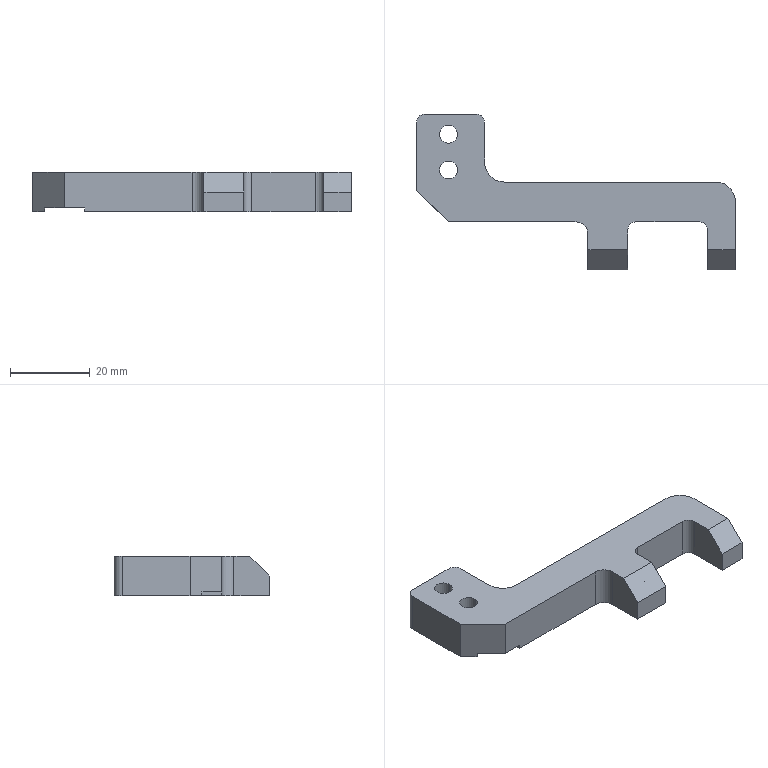Part | STEP file | PN_0045 | 1 solid | 48 faces | box 80 x 39 x 10 mm | volume 11727 mm3 | plane 21 | cylinder 19 | cone 8 | commonest cylinder face diameters 2.5 x8 4 x4 4.5 x4 10 x2 6 x1